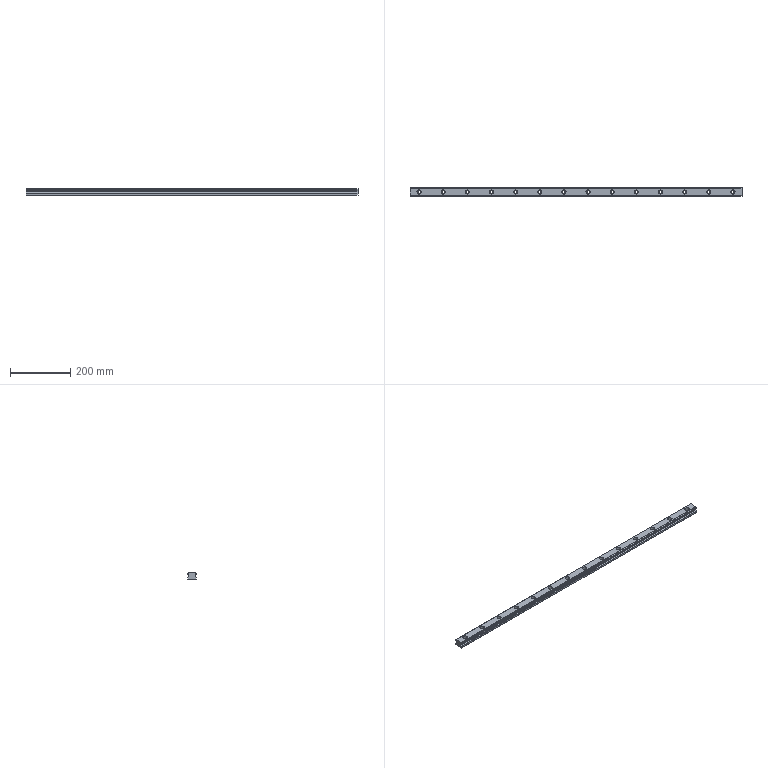Part | SolidWorks | features BaseBody 1 | 1 solid | 104 faces | box 1100 x 28 x 23 mm | volume 602385 mm3 | cylinder 74 | plane 30 | commonest cylinder face diameters 9 x28 14 x28 0.952 x2 0.976 x2 0.986 x2 0.995 x2